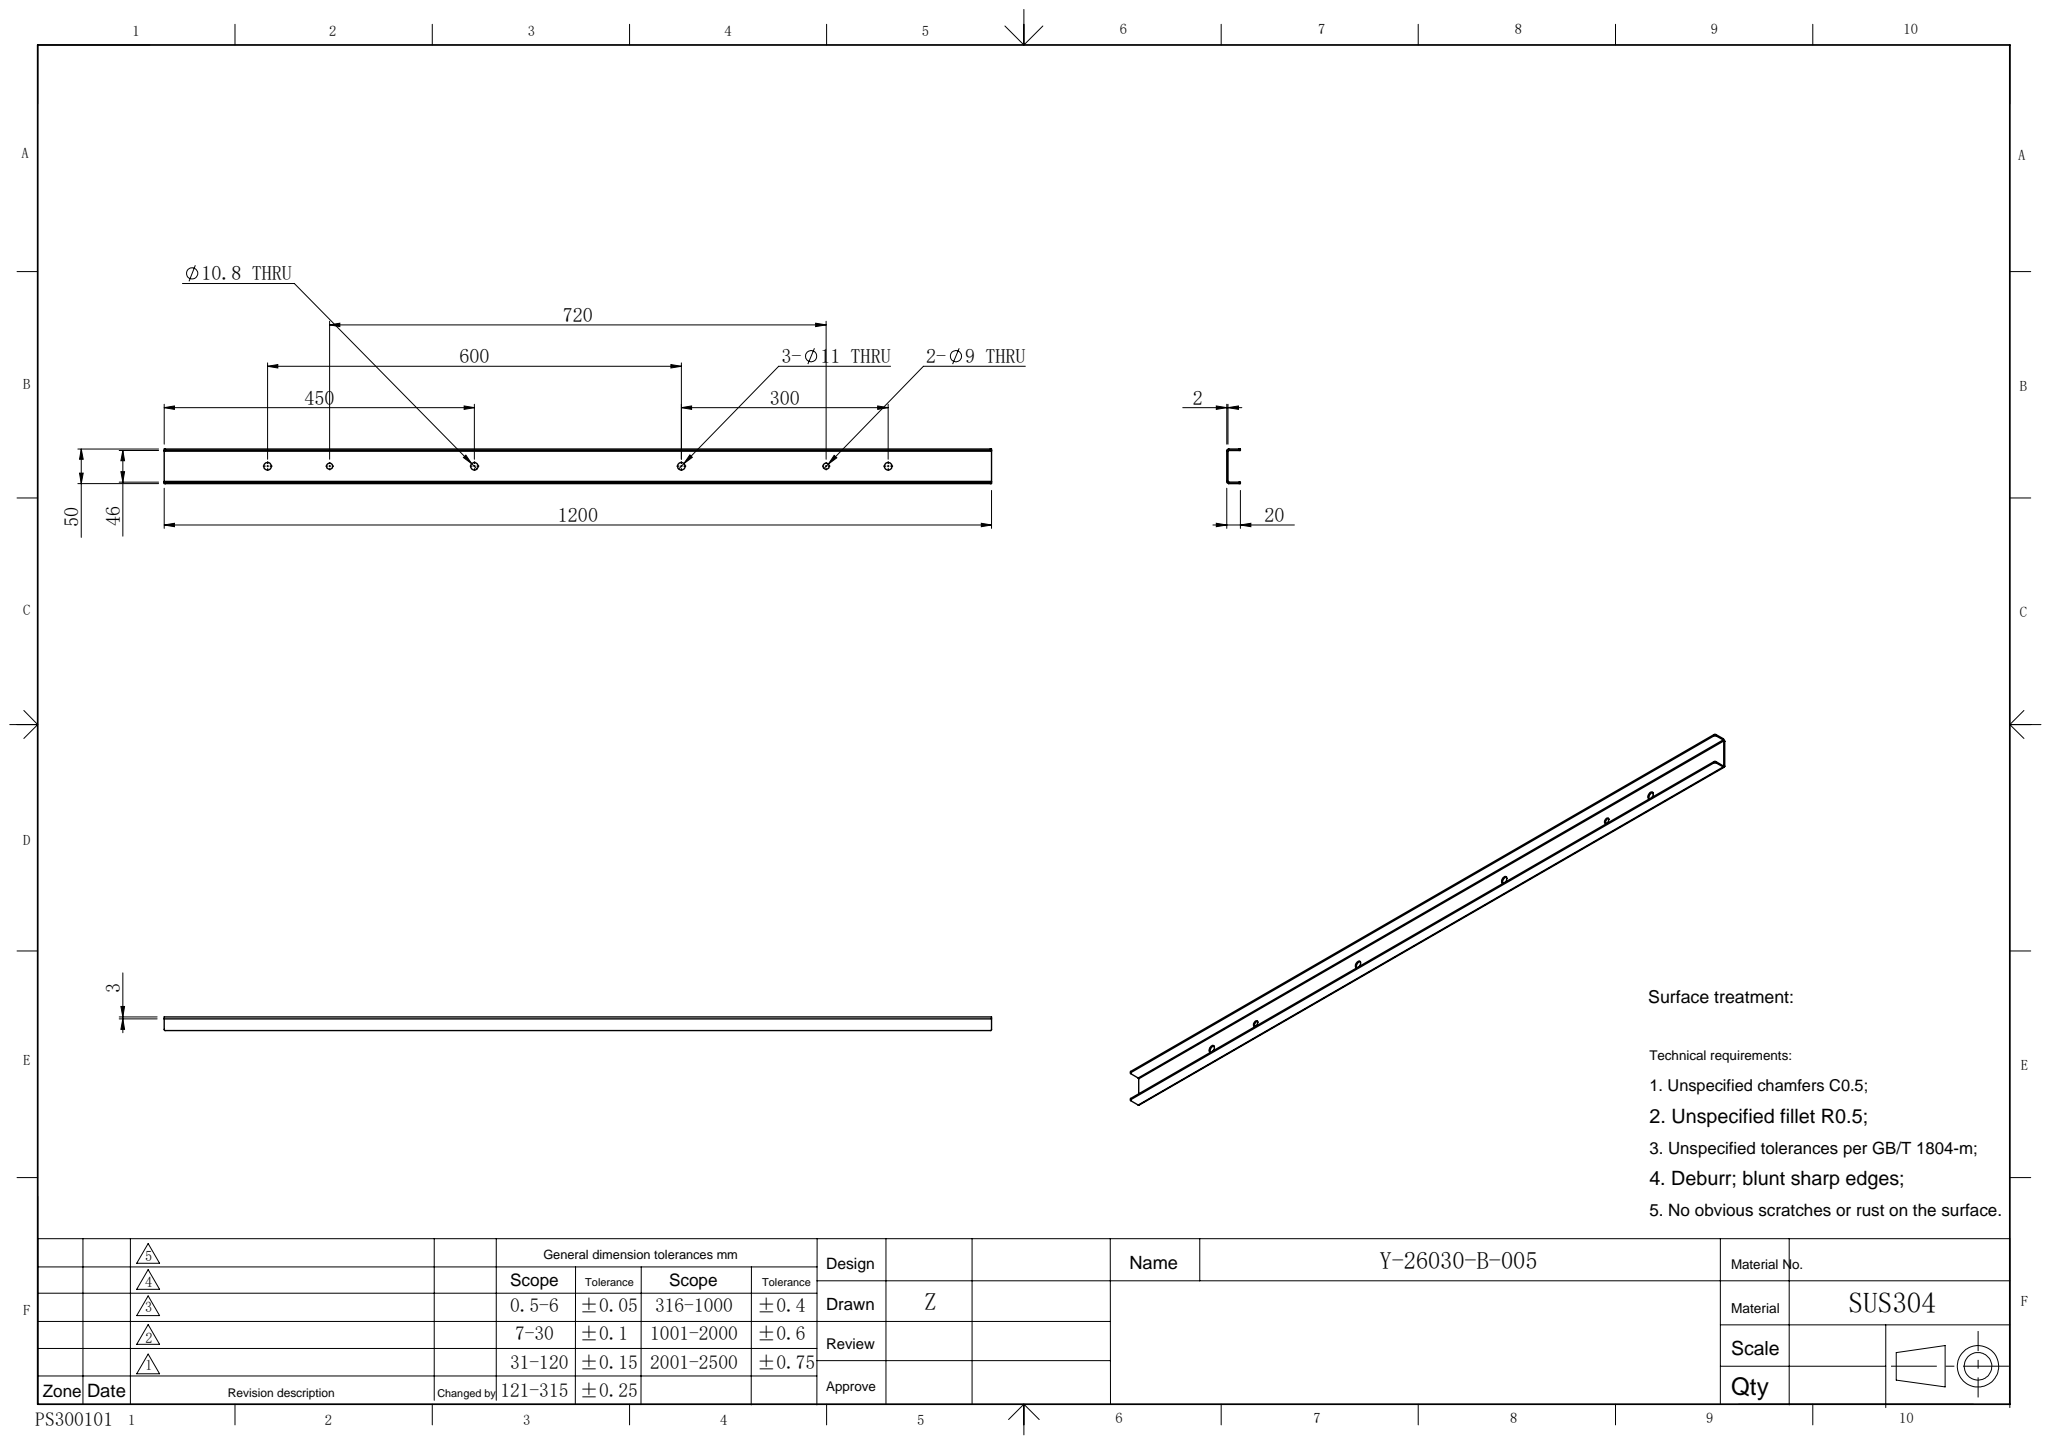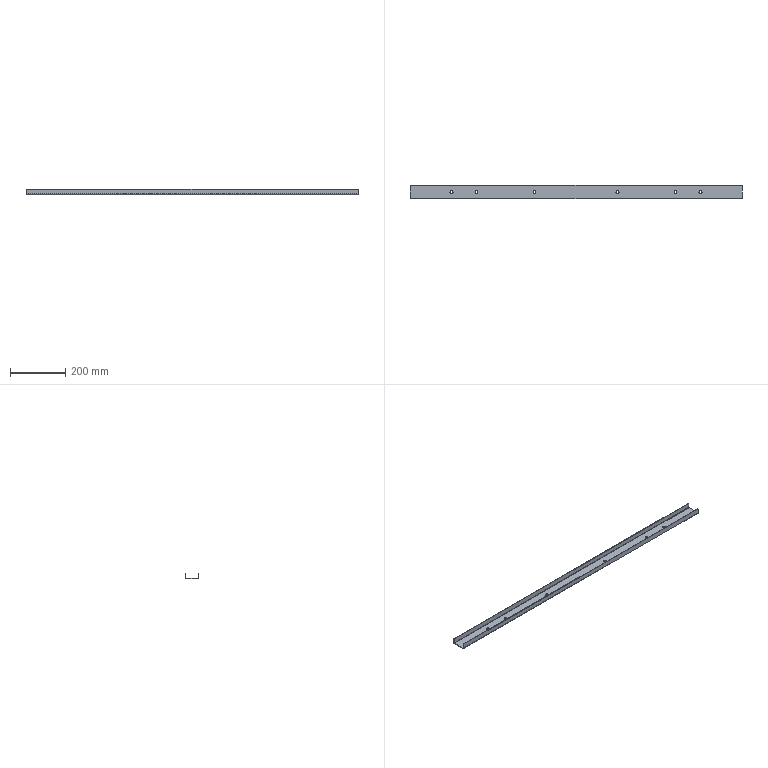Part | SolidWorks | features EdgeFlange 1, Fillet 1, FlatPattern 1, HoleWzd 1, ICE 1, SMBaseFlange 1, SheetMetal 1 | 1 solid | 38 faces | box 1200 x 50 x 20 mm | volume 201265 mm3 | cylinder 20 | plane 18 | commonest cylinder face diameters 11 x6 4 x4 9 x4 2 x2 6 x2 10.788 x2